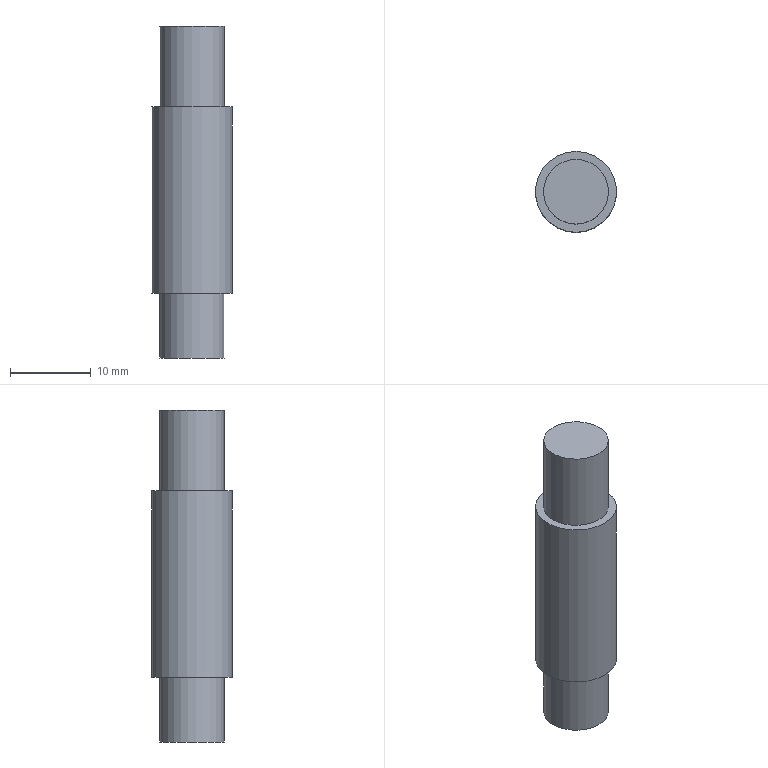Part | STEP file | 1-01.9 | 1 solid | 7 faces | box 10 x 10 x 41 mm | volume 2711 mm3 | plane 4 | cylinder 3 | commonest cylinder face diameters 8 x2 10 x1
STEP:
#1=CARTESIAN_POINT('',(0.,0.,0.));
#2=DIRECTION('',(0.,0.,1.));
#3=DIRECTION('',(1.,0.,0.));
#4=AXIS2_PLACEMENT_3D('',#1,#2,#3);
#5=CARTESIAN_POINT('',(0.,4.,10.));
#6=VERTEX_POINT('',#5);
#7=CARTESIAN_POINT('',(0.,0.,10.));
#8=DIRECTION('',(0.,0.,1.));
#9=DIRECTION('',(0.,1.,0.));
#10=AXIS2_PLACEMENT_3D('',#7,#8,#9);
#11=CIRCLE('',#10,4.);
#12=CARTESIAN_POINT('',(0.,-1.072,10.));
#13=DIRECTION('',(0.,0.,1.));
#14=DIRECTION('',(1.,0.,0.));
#15=AXIS2_PLACEMENT_3D('',#12,#13,#14);
#16=PLANE('',#15);
#17=CARTESIAN_POINT('',(0.,1.072));
#18=DIRECTION('',(0.,1.));
#19=AXIS2_PLACEMENT_2D('',#17,#18);
#20=CIRCLE('',#19,4.);
#21=(GEOMETRIC_REPRESENTATION_CONTEXT(2)PARAMETRIC_REPRESENTATION_CONTEXT()REPRESENTATION_CONTEXT('',''));
#22=DEFINITIONAL_REPRESENTATION('',(#20),#21);
#23=PCURVE('',#16,#22);
#24=CARTESIAN_POINT('',(0.,0.,0.));
#25=DIRECTION('',(0.,0.,1.));
#26=DIRECTION('',(0.,1.,0.));
#27=AXIS2_PLACEMENT_3D('',#24,#25,#26);
#28=CYLINDRICAL_SURFACE('',#27,4.);
#29=CARTESIAN_POINT('',(0.,10.));
#30=DIRECTION('',(1.,0.));
#31=VECTOR('',#30,1.);
#32=LINE('',#29,#31);
#33=(GEOMETRIC_REPRESENTATION_CONTEXT(2)PARAMETRIC_REPRESENTATION_CONTEXT()REPRESENTATION_CONTEXT('',''));
#34=DEFINITIONAL_REPRESENTATION('',(#32),#33);
#35=PCURVE('',#28,#34);
#36=SURFACE_CURVE('',#11,(#23,#35),.PCURVE_S1.);
#37=EDGE_CURVE('',#6,#6,#36,.T.);
#38=ORIENTED_EDGE('',*,*,#37,.T.);
#39=EDGE_LOOP('',(#38));
#40=FACE_BOUND('',#39,.T.);
#41=ADVANCED_FACE('',(#40),#16,.T.);
#42=CARTESIAN_POINT('',(0.,4.,0.));
#43=VERTEX_POINT('',#42);
#44=CARTESIAN_POINT('',(0.,0.,0.));
#45=DIRECTION('',(0.,0.,1.));
#46=DIRECTION('',(0.,1.,0.));
#47=AXIS2_PLACEMENT_3D('',#44,#45,#46);
#48=CIRCLE('',#47,4.);
#49=CARTESIAN_POINT('',(0.,0.));
#50=DIRECTION('',(1.,0.));
#51=VECTOR('',#50,1.);
#52=LINE('',#49,#51);
#53=(GEOMETRIC_REPRESENTATION_CONTEXT(2)PARAMETRIC_REPRESENTATION_CONTEXT()REPRESENTATION_CONTEXT('',''));
#54=DEFINITIONAL_REPRESENTATION('',(#52),#53);
#55=PCURVE('',#28,#54);
#56=CARTESIAN_POINT('',(0.,-1.34,0.));
#57=DIRECTION('',(0.,0.,1.));
#58=DIRECTION('',(1.,0.,0.));
#59=AXIS2_PLACEMENT_3D('',#56,#57,#58);
#60=PLANE('',#59);
#61=CARTESIAN_POINT('',(0.,1.34));
#62=DIRECTION('',(0.,1.));
#63=AXIS2_PLACEMENT_2D('',#61,#62);
#64=CIRCLE('',#63,4.);
#65=(GEOMETRIC_REPRESENTATION_CONTEXT(2)PARAMETRIC_REPRESENTATION_CONTEXT()REPRESENTATION_CONTEXT('',''));
#66=DEFINITIONAL_REPRESENTATION('',(#64),#65);
#67=PCURVE('',#60,#66);
#68=SURFACE_CURVE('',#48,(#55,#67),.PCURVE_S1.);
#69=EDGE_CURVE('',#43,#43,#68,.T.);
#70=ORIENTED_EDGE('',*,*,#69,.T.);
#71=CARTESIAN_POINT('',(0.,4.,0.));
#72=DIRECTION('',(0.,0.,1.));
#73=VECTOR('',#72,1.);
#74=LINE('',#71,#73);
#75=CARTESIAN_POINT('',(6.283,0.));
#76=DIRECTION('',(0.,1.));
#77=VECTOR('',#76,1.);
#78=LINE('',#75,#77);
#79=(GEOMETRIC_REPRESENTATION_CONTEXT(2)PARAMETRIC_REPRESENTATION_CONTEXT()REPRESENTATION_CONTEXT('',''));
#80=DEFINITIONAL_REPRESENTATION('',(#78),#79);
#81=PCURVE('',#28,#80);
#82=CARTESIAN_POINT('',(0.,0.));
#83=DIRECTION('',(0.,1.));
#84=VECTOR('',#83,1.);
#85=LINE('',#82,#84);
#86=(GEOMETRIC_REPRESENTATION_CONTEXT(2)PARAMETRIC_REPRESENTATION_CONTEXT()REPRESENTATION_CONTEXT('',''));
#87=DEFINITIONAL_REPRESENTATION('',(#85),#86);
#88=PCURVE('',#28,#87);
#89=SEAM_CURVE('',#74,(#81,#88),.PCURVE_S1.);
#90=EDGE_CURVE('',#43,#6,#89,.T.);
#91=ORIENTED_EDGE('',*,*,#90,.T.);
#92=ORIENTED_EDGE('',*,*,#37,.F.);
#93=ORIENTED_EDGE('',*,*,#90,.F.);
#94=EDGE_LOOP('',(#70,#91,#92,#93));
#95=FACE_BOUND('',#94,.T.);
#96=ADVANCED_FACE('',(#95),#28,.T.);
#97=CARTESIAN_POINT('',(0.,5.,0.));
#98=VERTEX_POINT('',#97);
#99=CARTESIAN_POINT('',(0.,0.,0.));
#100=DIRECTION('',(0.,0.,1.));
#101=DIRECTION('',(0.,1.,0.));
#102=AXIS2_PLACEMENT_3D('',#99,#100,#101);
#103=CIRCLE('',#102,5.);
#104=CARTESIAN_POINT('',(0.,1.34));
#105=DIRECTION('',(0.,1.));
#106=AXIS2_PLACEMENT_2D('',#104,#105);
#107=CIRCLE('',#106,5.);
#108=(GEOMETRIC_REPRESENTATION_CONTEXT(2)PARAMETRIC_REPRESENTATION_CONTEXT()REPRESENTATION_CONTEXT('',''));
#109=DEFINITIONAL_REPRESENTATION('',(#107),#108);
#110=PCURVE('',#60,#109);
#111=CARTESIAN_POINT('',(0.,0.,0.));
#112=DIRECTION('',(0.,0.,-1.));
#113=DIRECTION('',(0.,1.,0.));
#114=AXIS2_PLACEMENT_3D('',#111,#112,#113);
#115=CYLINDRICAL_SURFACE('',#114,5.);
#116=CARTESIAN_POINT('',(6.283,0.));
#117=DIRECTION('',(-1.,0.));
#118=VECTOR('',#117,1.);
#119=LINE('',#116,#118);
#120=(GEOMETRIC_REPRESENTATION_CONTEXT(2)PARAMETRIC_REPRESENTATION_CONTEXT()REPRESENTATION_CONTEXT('',''));
#121=DEFINITIONAL_REPRESENTATION('',(#119),#120);
#122=PCURVE('',#115,#121);
#123=SURFACE_CURVE('',#103,(#110,#122),.PCURVE_S1.);
#124=EDGE_CURVE('',#98,#98,#123,.T.);
#125=ORIENTED_EDGE('',*,*,#124,.T.);
#126=EDGE_LOOP('',(#125));
#127=FACE_BOUND('',#126,.T.);
#128=ORIENTED_EDGE('',*,*,#69,.F.);
#129=EDGE_LOOP('',(#128));
#130=FACE_BOUND('',#129,.T.);
#131=ADVANCED_FACE('',(#127,#130),#60,.T.);
#132=CARTESIAN_POINT('',(0.,5.,-23.));
#133=VERTEX_POINT('',#132);
#134=CARTESIAN_POINT('',(0.,5.,0.));
#135=DIRECTION('',(0.,0.,-1.));
#136=VECTOR('',#135,1.);
#137=LINE('',#134,#136);
#138=CARTESIAN_POINT('',(6.283,0.));
#139=DIRECTION('',(0.,1.));
#140=VECTOR('',#139,1.);
#141=LINE('',#138,#140);
#142=(GEOMETRIC_REPRESENTATION_CONTEXT(2)PARAMETRIC_REPRESENTATION_CONTEXT()REPRESENTATION_CONTEXT('',''));
#143=DEFINITIONAL_REPRESENTATION('',(#141),#142);
#144=PCURVE('',#115,#143);
#145=CARTESIAN_POINT('',(0.,0.));
#146=DIRECTION('',(0.,1.));
#147=VECTOR('',#146,1.);
#148=LINE('',#145,#147);
#149=(GEOMETRIC_REPRESENTATION_CONTEXT(2)PARAMETRIC_REPRESENTATION_CONTEXT()REPRESENTATION_CONTEXT('',''));
#150=DEFINITIONAL_REPRESENTATION('',(#148),#149);
#151=PCURVE('',#115,#150);
#152=SEAM_CURVE('',#137,(#144,#151),.PCURVE_S1.);
#153=EDGE_CURVE('',#98,#133,#152,.T.);
#154=ORIENTED_EDGE('',*,*,#153,.T.);
#155=CARTESIAN_POINT('',(0.,0.,-23.));
#156=DIRECTION('',(0.,0.,1.));
#157=DIRECTION('',(0.,1.,0.));
#158=AXIS2_PLACEMENT_3D('',#155,#156,#157);
#159=CIRCLE('',#158,5.);
#160=CARTESIAN_POINT('',(6.283,23.));
#161=DIRECTION('',(-1.,0.));
#162=VECTOR('',#161,1.);
#163=LINE('',#160,#162);
#164=(GEOMETRIC_REPRESENTATION_CONTEXT(2)PARAMETRIC_REPRESENTATION_CONTEXT()REPRESENTATION_CONTEXT('',''));
#165=DEFINITIONAL_REPRESENTATION('',(#163),#164);
#166=PCURVE('',#115,#165);
#167=CARTESIAN_POINT('',(0.,-1.34,-23.));
#168=DIRECTION('',(0.,0.,1.));
#169=DIRECTION('',(1.,0.,0.));
#170=AXIS2_PLACEMENT_3D('',#167,#168,#169);
#171=PLANE('',#170);
#172=CARTESIAN_POINT('',(0.,1.34));
#173=DIRECTION('',(0.,1.));
#174=AXIS2_PLACEMENT_2D('',#172,#173);
#175=CIRCLE('',#174,5.);
#176=(GEOMETRIC_REPRESENTATION_CONTEXT(2)PARAMETRIC_REPRESENTATION_CONTEXT()REPRESENTATION_CONTEXT('',''));
#177=DEFINITIONAL_REPRESENTATION('',(#175),#176);
#178=PCURVE('',#171,#177);
#179=SURFACE_CURVE('',#159,(#166,#178),.PCURVE_S1.);
#180=EDGE_CURVE('',#133,#133,#179,.T.);
#181=ORIENTED_EDGE('',*,*,#180,.T.);
#182=ORIENTED_EDGE('',*,*,#153,.F.);
#183=ORIENTED_EDGE('',*,*,#124,.F.);
#184=EDGE_LOOP('',(#154,#181,#182,#183));
#185=FACE_BOUND('',#184,.T.);
#186=ADVANCED_FACE('',(#185),#115,.T.);
#187=ORIENTED_EDGE('',*,*,#180,.T.);
#188=EDGE_LOOP('',(#187));
#189=FACE_BOUND('',#188,.F.);
#190=CARTESIAN_POINT('',(0.,4.,-23.));
#191=VERTEX_POINT('',#190);
#192=CARTESIAN_POINT('',(0.,0.,-23.));
#193=DIRECTION('',(0.,0.,-1.));
#194=DIRECTION('',(0.,1.,0.));
#195=AXIS2_PLACEMENT_3D('',#192,#193,#194);
#196=CIRCLE('',#195,4.);
#197=CARTESIAN_POINT('',(0.,5.34));
#198=CARTESIAN_POINT('',(6.928,5.34));
#199=CARTESIAN_POINT('',(3.464,-0.6603));
#200=CARTESIAN_POINT('',(0.,-6.66));
#201=CARTESIAN_POINT('',(-3.464,-0.6603));
#202=CARTESIAN_POINT('',(-6.928,5.34));
#203=CARTESIAN_POINT('',(0.,5.34));
#204=(BOUNDED_CURVE()B_SPLINE_CURVE(2,(#197,#198,#199,#200,#201,#202,#203),.UNSPECIFIED.,.T.,.F.)B_SPLINE_CURVE_WITH_KNOTS((1,2,2,2,2,1),(-2.094,0.,2.094,4.189,6.283,8.378),.UNSPECIFIED.)CURVE()GEOMETRIC_REPRESENTATION_ITEM()RATIONAL_B_SPLINE_CURVE((1.,0.5,1.,0.5,1.,0.5,1.))REPRESENTATION_ITEM(''));
#205=(GEOMETRIC_REPRESENTATION_CONTEXT(2)PARAMETRIC_REPRESENTATION_CONTEXT()REPRESENTATION_CONTEXT('',''));
#206=DEFINITIONAL_REPRESENTATION('',(#204),#205);
#207=PCURVE('',#171,#206);
#208=CARTESIAN_POINT('',(0.,0.,-23.));
#209=DIRECTION('',(0.,0.,-1.));
#210=DIRECTION('',(0.,1.,0.));
#211=AXIS2_PLACEMENT_3D('',#208,#209,#210);
#212=CYLINDRICAL_SURFACE('',#211,4.);
#213=CARTESIAN_POINT('',(0.,0.));
#214=DIRECTION('',(1.,0.));
#215=VECTOR('',#214,1.);
#216=LINE('',#213,#215);
#217=(GEOMETRIC_REPRESENTATION_CONTEXT(2)PARAMETRIC_REPRESENTATION_CONTEXT()REPRESENTATION_CONTEXT('',''));
#218=DEFINITIONAL_REPRESENTATION('',(#216),#217);
#219=PCURVE('',#212,#218);
#220=SURFACE_CURVE('',#196,(#207,#219),.PCURVE_S1.);
#221=EDGE_CURVE('',#191,#191,#220,.T.);
#222=ORIENTED_EDGE('',*,*,#221,.T.);
#223=EDGE_LOOP('',(#222));
#224=FACE_BOUND('',#223,.F.);
#225=ADVANCED_FACE('',(#189,#224),#171,.F.);
#226=ORIENTED_EDGE('',*,*,#221,.T.);
#227=CARTESIAN_POINT('',(0.,4.,-31.));
#228=VERTEX_POINT('',#227);
#229=CARTESIAN_POINT('',(0.,4.,-23.));
#230=DIRECTION('',(0.,0.,-1.));
#231=VECTOR('',#230,1.);
#232=LINE('',#229,#231);
#233=CARTESIAN_POINT('',(6.283,0.));
#234=DIRECTION('',(0.,1.));
#235=VECTOR('',#234,1.);
#236=LINE('',#233,#235);
#237=(GEOMETRIC_REPRESENTATION_CONTEXT(2)PARAMETRIC_REPRESENTATION_CONTEXT()REPRESENTATION_CONTEXT('',''));
#238=DEFINITIONAL_REPRESENTATION('',(#236),#237);
#239=PCURVE('',#212,#238);
#240=CARTESIAN_POINT('',(0.,0.));
#241=DIRECTION('',(0.,1.));
#242=VECTOR('',#241,1.);
#243=LINE('',#240,#242);
#244=(GEOMETRIC_REPRESENTATION_CONTEXT(2)PARAMETRIC_REPRESENTATION_CONTEXT()REPRESENTATION_CONTEXT('',''));
#245=DEFINITIONAL_REPRESENTATION('',(#243),#244);
#246=PCURVE('',#212,#245);
#247=SEAM_CURVE('',#232,(#239,#246),.PCURVE_S1.);
#248=EDGE_CURVE('',#191,#228,#247,.T.);
#249=ORIENTED_EDGE('',*,*,#248,.T.);
#250=CARTESIAN_POINT('',(0.,0.,-31.));
#251=DIRECTION('',(0.,0.,-1.));
#252=DIRECTION('',(0.,1.,0.));
#253=AXIS2_PLACEMENT_3D('',#250,#251,#252);
#254=CIRCLE('',#253,4.);
#255=CARTESIAN_POINT('',(0.,8.));
#256=DIRECTION('',(1.,0.));
#257=VECTOR('',#256,1.);
#258=LINE('',#255,#257);
#259=(GEOMETRIC_REPRESENTATION_CONTEXT(2)PARAMETRIC_REPRESENTATION_CONTEXT()REPRESENTATION_CONTEXT('',''));
#260=DEFINITIONAL_REPRESENTATION('',(#258),#259);
#261=PCURVE('',#212,#260);
#262=CARTESIAN_POINT('',(0.,-1.072,-31.));
#263=DIRECTION('',(0.,0.,-1.));
#264=DIRECTION('',(0.,1.,0.));
#265=AXIS2_PLACEMENT_3D('',#262,#263,#264);
#266=PLANE('',#265);
#267=CARTESIAN_POINT('',(1.072,0.));
#268=DIRECTION('',(1.,0.));
#269=AXIS2_PLACEMENT_2D('',#267,#268);
#270=CIRCLE('',#269,4.);
#271=(GEOMETRIC_REPRESENTATION_CONTEXT(2)PARAMETRIC_REPRESENTATION_CONTEXT()REPRESENTATION_CONTEXT('',''));
#272=DEFINITIONAL_REPRESENTATION('',(#270),#271);
#273=PCURVE('',#266,#272);
#274=SURFACE_CURVE('',#254,(#261,#273),.PCURVE_S1.);
#275=EDGE_CURVE('',#228,#228,#274,.T.);
#276=ORIENTED_EDGE('',*,*,#275,.F.);
#277=ORIENTED_EDGE('',*,*,#248,.F.);
#278=EDGE_LOOP('',(#226,#249,#276,#277));
#279=FACE_BOUND('',#278,.T.);
#280=ADVANCED_FACE('',(#279),#212,.T.);
#281=ORIENTED_EDGE('',*,*,#275,.T.);
#282=EDGE_LOOP('',(#281));
#283=FACE_BOUND('',#282,.T.);
#284=ADVANCED_FACE('',(#283),#266,.T.);
#285=CLOSED_SHELL('',(#41,#96,#131,#186,#225,#280,#284));
#286=MANIFOLD_SOLID_BREP('',#285);
#287=(LENGTH_UNIT()NAMED_UNIT(*)SI_UNIT(.MILLI.,.METRE.));
#288=UNCERTAINTY_MEASURE_WITH_UNIT(LENGTH_MEASURE(0.0000001),#287,'','');
#289=(NAMED_UNIT(*)PLANE_ANGLE_UNIT()SI_UNIT($,.RADIAN.));
#290=(NAMED_UNIT(*)SI_UNIT($,.STERADIAN.)SOLID_ANGLE_UNIT());
#291=(GEOMETRIC_REPRESENTATION_CONTEXT(3)GLOBAL_UNCERTAINTY_ASSIGNED_CONTEXT((#288))GLOBAL_UNIT_ASSIGNED_CONTEXT((#287,#289,#290))REPRESENTATION_CONTEXT('',''));
#292=ADVANCED_BREP_SHAPE_REPRESENTATION('',(#4,#286),#291);